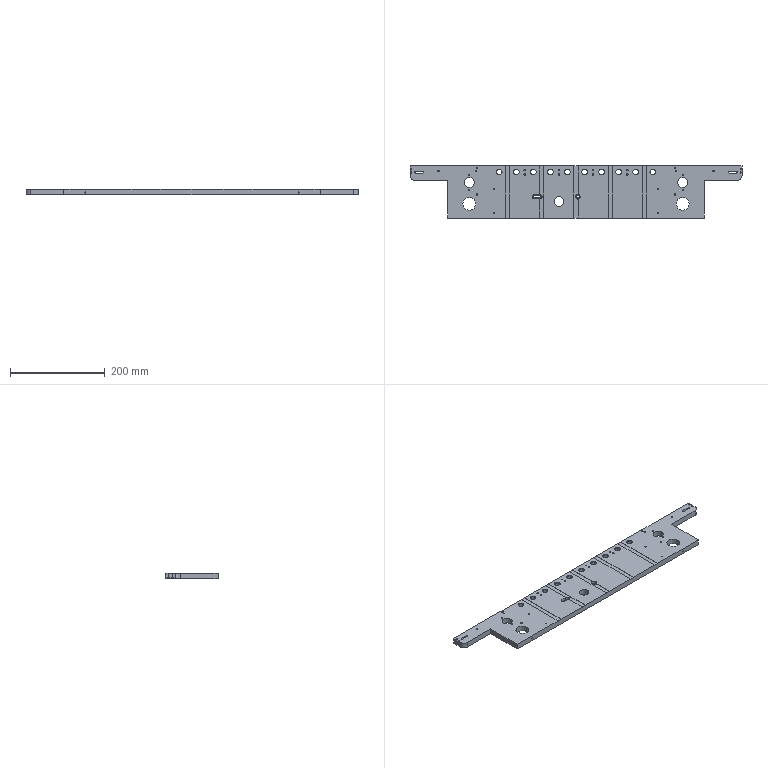Part | SolidWorks | features HoleWzd 12, ICE 7, Extrusion 1, Fillet 1, LPattern 1 | 1 solid | 236 faces | box 700 x 110 x 12 mm | volume 712191 mm3 | cylinder 172 | plane 56 | cone 8 | commonest cylinder face diameters 2.5 x48 3.3 x40 12 x20 16 x20 2.4 x8 4.3 x8